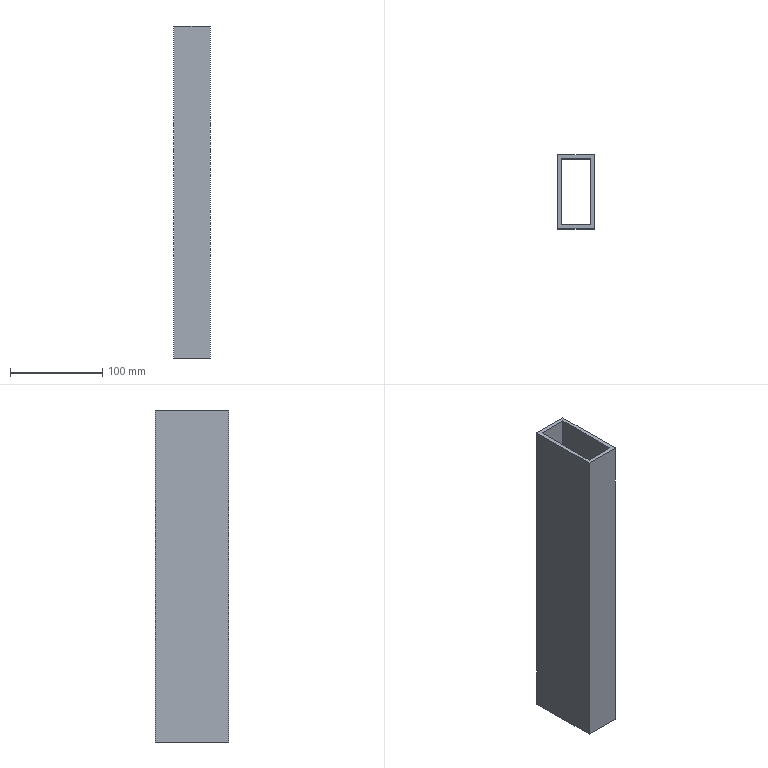Part | SolidWorks | features Extrusion 1 | 1 solid | 10 faces | box 40 x 80 x 360 mm | volume 322560 mm3 | plane 10
STEP:
#1=CARTESIAN_POINT('',(-20.,40.,180.));
#2=VERTEX_POINT('',#1);
#3=CARTESIAN_POINT('',(-20.,-40.,180.));
#4=VERTEX_POINT('',#3);
#5=CARTESIAN_POINT('',(-20.,40.,180.));
#6=DIRECTION('',(0.,-1.,0.));
#7=VECTOR('',#6,1000.);
#8=LINE('',#5,#7);
#9=EDGE_CURVE('',#2,#4,#8,.T.);
#10=ORIENTED_EDGE('',*,*,#9,.F.);
#11=CARTESIAN_POINT('',(-20.,40.,-180.));
#12=VERTEX_POINT('',#11);
#13=CARTESIAN_POINT('',(-20.,40.,-180.));
#14=DIRECTION('',(0.,0.,1.));
#15=VECTOR('',#14,1000.);
#16=LINE('',#13,#15);
#17=EDGE_CURVE('',#12,#2,#16,.T.);
#18=ORIENTED_EDGE('',*,*,#17,.F.);
#19=CARTESIAN_POINT('',(-20.,-40.,-180.));
#20=VERTEX_POINT('',#19);
#21=CARTESIAN_POINT('',(-20.,40.,-180.));
#22=DIRECTION('',(0.,-1.,0.));
#23=VECTOR('',#22,1000.);
#24=LINE('',#21,#23);
#25=EDGE_CURVE('',#12,#20,#24,.T.);
#26=ORIENTED_EDGE('',*,*,#25,.T.);
#27=CARTESIAN_POINT('',(-20.,-40.,-180.));
#28=DIRECTION('',(0.,0.,1.));
#29=VECTOR('',#28,1000.);
#30=LINE('',#27,#29);
#31=EDGE_CURVE('',#20,#4,#30,.T.);
#32=ORIENTED_EDGE('',*,*,#31,.T.);
#33=EDGE_LOOP('',(#10,#18,#26,#32));
#34=FACE_OUTER_BOUND('',#33,.T.);
#35=CARTESIAN_POINT('',(-20.,40.,-180.));
#36=DIRECTION('',(-1.,0.,0.));
#37=DIRECTION('',(0.,0.,1.));
#38=AXIS2_PLACEMENT_3D('',#35,#36,#37);
#39=PLANE('',#38);
#40=ADVANCED_FACE('',(#34),#39,.T.);
#41=CARTESIAN_POINT('',(20.,40.,180.));
#42=VERTEX_POINT('',#41);
#43=CARTESIAN_POINT('',(20.,40.,180.));
#44=DIRECTION('',(-1.,0.,0.));
#45=VECTOR('',#44,1000.);
#46=LINE('',#43,#45);
#47=EDGE_CURVE('',#42,#2,#46,.T.);
#48=ORIENTED_EDGE('',*,*,#47,.F.);
#49=CARTESIAN_POINT('',(20.,40.,-180.));
#50=VERTEX_POINT('',#49);
#51=CARTESIAN_POINT('',(20.,40.,-180.));
#52=DIRECTION('',(0.,0.,1.));
#53=VECTOR('',#52,1000.);
#54=LINE('',#51,#53);
#55=EDGE_CURVE('',#50,#42,#54,.T.);
#56=ORIENTED_EDGE('',*,*,#55,.F.);
#57=CARTESIAN_POINT('',(20.,40.,-180.));
#58=DIRECTION('',(-1.,0.,0.));
#59=VECTOR('',#58,1000.);
#60=LINE('',#57,#59);
#61=EDGE_CURVE('',#50,#12,#60,.T.);
#62=ORIENTED_EDGE('',*,*,#61,.T.);
#63=ORIENTED_EDGE('',*,*,#17,.T.);
#64=EDGE_LOOP('',(#48,#56,#62,#63));
#65=FACE_OUTER_BOUND('',#64,.T.);
#66=CARTESIAN_POINT('',(20.,40.,-180.));
#67=DIRECTION('',(0.,1.,0.));
#68=DIRECTION('',(0.,0.,1.));
#69=AXIS2_PLACEMENT_3D('',#66,#67,#68);
#70=PLANE('',#69);
#71=ADVANCED_FACE('',(#65),#70,.T.);
#72=CARTESIAN_POINT('',(20.,-40.,180.));
#73=VERTEX_POINT('',#72);
#74=CARTESIAN_POINT('',(20.,-40.,180.));
#75=DIRECTION('',(0.,1.,0.));
#76=VECTOR('',#75,1000.);
#77=LINE('',#74,#76);
#78=EDGE_CURVE('',#73,#42,#77,.T.);
#79=ORIENTED_EDGE('',*,*,#78,.F.);
#80=CARTESIAN_POINT('',(20.,-40.,-180.));
#81=VERTEX_POINT('',#80);
#82=CARTESIAN_POINT('',(20.,-40.,-180.));
#83=DIRECTION('',(0.,0.,1.));
#84=VECTOR('',#83,1000.);
#85=LINE('',#82,#84);
#86=EDGE_CURVE('',#81,#73,#85,.T.);
#87=ORIENTED_EDGE('',*,*,#86,.F.);
#88=CARTESIAN_POINT('',(20.,-40.,-180.));
#89=DIRECTION('',(0.,1.,0.));
#90=VECTOR('',#89,1000.);
#91=LINE('',#88,#90);
#92=EDGE_CURVE('',#81,#50,#91,.T.);
#93=ORIENTED_EDGE('',*,*,#92,.T.);
#94=ORIENTED_EDGE('',*,*,#55,.T.);
#95=EDGE_LOOP('',(#79,#87,#93,#94));
#96=FACE_OUTER_BOUND('',#95,.T.);
#97=CARTESIAN_POINT('',(20.,-40.,-180.));
#98=DIRECTION('',(1.,0.,0.));
#99=DIRECTION('',(0.,0.,-1.));
#100=AXIS2_PLACEMENT_3D('',#97,#98,#99);
#101=PLANE('',#100);
#102=ADVANCED_FACE('',(#96),#101,.T.);
#103=CARTESIAN_POINT('',(-20.,-40.,180.));
#104=DIRECTION('',(1.,0.,0.));
#105=VECTOR('',#104,1000.);
#106=LINE('',#103,#105);
#107=EDGE_CURVE('',#4,#73,#106,.T.);
#108=ORIENTED_EDGE('',*,*,#107,.F.);
#109=ORIENTED_EDGE('',*,*,#31,.F.);
#110=CARTESIAN_POINT('',(-20.,-40.,-180.));
#111=DIRECTION('',(1.,0.,0.));
#112=VECTOR('',#111,1000.);
#113=LINE('',#110,#112);
#114=EDGE_CURVE('',#20,#81,#113,.T.);
#115=ORIENTED_EDGE('',*,*,#114,.T.);
#116=ORIENTED_EDGE('',*,*,#86,.T.);
#117=EDGE_LOOP('',(#108,#109,#115,#116));
#118=FACE_OUTER_BOUND('',#117,.T.);
#119=CARTESIAN_POINT('',(-20.,-40.,-180.));
#120=DIRECTION('',(0.,-1.,0.));
#121=DIRECTION('',(0.,0.,-1.));
#122=AXIS2_PLACEMENT_3D('',#119,#120,#121);
#123=PLANE('',#122);
#124=ADVANCED_FACE('',(#118),#123,.T.);
#125=CARTESIAN_POINT('',(16.,36.,-180.));
#126=VERTEX_POINT('',#125);
#127=CARTESIAN_POINT('',(-16.,36.,-180.));
#128=VERTEX_POINT('',#127);
#129=CARTESIAN_POINT('',(16.,36.,-180.));
#130=DIRECTION('',(-1.,0.,0.));
#131=VECTOR('',#130,1000.);
#132=LINE('',#129,#131);
#133=EDGE_CURVE('',#126,#128,#132,.T.);
#134=ORIENTED_EDGE('',*,*,#133,.T.);
#135=CARTESIAN_POINT('',(-16.,-36.,-180.));
#136=VERTEX_POINT('',#135);
#137=CARTESIAN_POINT('',(-16.,36.,-180.));
#138=DIRECTION('',(0.,-1.,0.));
#139=VECTOR('',#138,1000.);
#140=LINE('',#137,#139);
#141=EDGE_CURVE('',#128,#136,#140,.T.);
#142=ORIENTED_EDGE('',*,*,#141,.T.);
#143=CARTESIAN_POINT('',(16.,-36.,-180.));
#144=VERTEX_POINT('',#143);
#145=CARTESIAN_POINT('',(-16.,-36.,-180.));
#146=DIRECTION('',(1.,0.,0.));
#147=VECTOR('',#146,1000.);
#148=LINE('',#145,#147);
#149=EDGE_CURVE('',#136,#144,#148,.T.);
#150=ORIENTED_EDGE('',*,*,#149,.T.);
#151=CARTESIAN_POINT('',(16.,-36.,-180.));
#152=DIRECTION('',(0.,1.,0.));
#153=VECTOR('',#152,1000.);
#154=LINE('',#151,#153);
#155=EDGE_CURVE('',#144,#126,#154,.T.);
#156=ORIENTED_EDGE('',*,*,#155,.T.);
#157=EDGE_LOOP('',(#134,#142,#150,#156));
#158=FACE_BOUND('',#157,.T.);
#159=ORIENTED_EDGE('',*,*,#25,.F.);
#160=ORIENTED_EDGE('',*,*,#61,.F.);
#161=ORIENTED_EDGE('',*,*,#92,.F.);
#162=ORIENTED_EDGE('',*,*,#114,.F.);
#163=EDGE_LOOP('',(#159,#160,#161,#162));
#164=FACE_OUTER_BOUND('',#163,.T.);
#165=CARTESIAN_POINT('',(0.,0.,-180.));
#166=DIRECTION('',(0.,0.,1.));
#167=DIRECTION('',(1.,0.,0.));
#168=AXIS2_PLACEMENT_3D('',#165,#166,#167);
#169=PLANE('',#168);
#170=ADVANCED_FACE('',(#158,#164),#169,.F.);
#171=CARTESIAN_POINT('',(-16.,36.,180.));
#172=VERTEX_POINT('',#171);
#173=CARTESIAN_POINT('',(-16.,-36.,180.));
#174=VERTEX_POINT('',#173);
#175=CARTESIAN_POINT('',(-16.,36.,180.));
#176=DIRECTION('',(0.,-1.,0.));
#177=VECTOR('',#176,1000.);
#178=LINE('',#175,#177);
#179=EDGE_CURVE('',#172,#174,#178,.T.);
#180=ORIENTED_EDGE('',*,*,#179,.F.);
#181=CARTESIAN_POINT('',(16.,36.,180.));
#182=VERTEX_POINT('',#181);
#183=CARTESIAN_POINT('',(16.,36.,180.));
#184=DIRECTION('',(-1.,0.,0.));
#185=VECTOR('',#184,1000.);
#186=LINE('',#183,#185);
#187=EDGE_CURVE('',#182,#172,#186,.T.);
#188=ORIENTED_EDGE('',*,*,#187,.F.);
#189=CARTESIAN_POINT('',(16.,-36.,180.));
#190=VERTEX_POINT('',#189);
#191=CARTESIAN_POINT('',(16.,-36.,180.));
#192=DIRECTION('',(0.,1.,0.));
#193=VECTOR('',#192,1000.);
#194=LINE('',#191,#193);
#195=EDGE_CURVE('',#190,#182,#194,.T.);
#196=ORIENTED_EDGE('',*,*,#195,.F.);
#197=CARTESIAN_POINT('',(-16.,-36.,180.));
#198=DIRECTION('',(1.,0.,0.));
#199=VECTOR('',#198,1000.);
#200=LINE('',#197,#199);
#201=EDGE_CURVE('',#174,#190,#200,.T.);
#202=ORIENTED_EDGE('',*,*,#201,.F.);
#203=EDGE_LOOP('',(#180,#188,#196,#202));
#204=FACE_BOUND('',#203,.T.);
#205=ORIENTED_EDGE('',*,*,#9,.T.);
#206=ORIENTED_EDGE('',*,*,#107,.T.);
#207=ORIENTED_EDGE('',*,*,#78,.T.);
#208=ORIENTED_EDGE('',*,*,#47,.T.);
#209=EDGE_LOOP('',(#205,#206,#207,#208));
#210=FACE_OUTER_BOUND('',#209,.T.);
#211=CARTESIAN_POINT('',(0.,0.,180.));
#212=DIRECTION('',(0.,0.,1.));
#213=DIRECTION('',(1.,0.,0.));
#214=AXIS2_PLACEMENT_3D('',#211,#212,#213);
#215=PLANE('',#214);
#216=ADVANCED_FACE('',(#204,#210),#215,.T.);
#217=ORIENTED_EDGE('',*,*,#179,.T.);
#218=CARTESIAN_POINT('',(-16.,-36.,-180.));
#219=DIRECTION('',(0.,0.,1.));
#220=VECTOR('',#219,1000.);
#221=LINE('',#218,#220);
#222=EDGE_CURVE('',#136,#174,#221,.T.);
#223=ORIENTED_EDGE('',*,*,#222,.F.);
#224=ORIENTED_EDGE('',*,*,#141,.F.);
#225=CARTESIAN_POINT('',(-16.,36.,-180.));
#226=DIRECTION('',(0.,0.,1.));
#227=VECTOR('',#226,1000.);
#228=LINE('',#225,#227);
#229=EDGE_CURVE('',#128,#172,#228,.T.);
#230=ORIENTED_EDGE('',*,*,#229,.T.);
#231=EDGE_LOOP('',(#217,#223,#224,#230));
#232=FACE_OUTER_BOUND('',#231,.T.);
#233=CARTESIAN_POINT('',(-16.,36.,-180.));
#234=DIRECTION('',(-1.,0.,0.));
#235=DIRECTION('',(0.,0.,1.));
#236=AXIS2_PLACEMENT_3D('',#233,#234,#235);
#237=PLANE('',#236);
#238=ADVANCED_FACE('',(#232),#237,.F.);
#239=ORIENTED_EDGE('',*,*,#187,.T.);
#240=ORIENTED_EDGE('',*,*,#229,.F.);
#241=ORIENTED_EDGE('',*,*,#133,.F.);
#242=CARTESIAN_POINT('',(16.,36.,-180.));
#243=DIRECTION('',(0.,0.,1.));
#244=VECTOR('',#243,1000.);
#245=LINE('',#242,#244);
#246=EDGE_CURVE('',#126,#182,#245,.T.);
#247=ORIENTED_EDGE('',*,*,#246,.T.);
#248=EDGE_LOOP('',(#239,#240,#241,#247));
#249=FACE_OUTER_BOUND('',#248,.T.);
#250=CARTESIAN_POINT('',(16.,36.,-180.));
#251=DIRECTION('',(0.,1.,0.));
#252=DIRECTION('',(0.,0.,1.));
#253=AXIS2_PLACEMENT_3D('',#250,#251,#252);
#254=PLANE('',#253);
#255=ADVANCED_FACE('',(#249),#254,.F.);
#256=ORIENTED_EDGE('',*,*,#195,.T.);
#257=ORIENTED_EDGE('',*,*,#246,.F.);
#258=ORIENTED_EDGE('',*,*,#155,.F.);
#259=CARTESIAN_POINT('',(16.,-36.,-180.));
#260=DIRECTION('',(0.,0.,1.));
#261=VECTOR('',#260,1000.);
#262=LINE('',#259,#261);
#263=EDGE_CURVE('',#144,#190,#262,.T.);
#264=ORIENTED_EDGE('',*,*,#263,.T.);
#265=EDGE_LOOP('',(#256,#257,#258,#264));
#266=FACE_OUTER_BOUND('',#265,.T.);
#267=CARTESIAN_POINT('',(16.,-36.,-180.));
#268=DIRECTION('',(1.,0.,0.));
#269=DIRECTION('',(0.,0.,-1.));
#270=AXIS2_PLACEMENT_3D('',#267,#268,#269);
#271=PLANE('',#270);
#272=ADVANCED_FACE('',(#266),#271,.F.);
#273=ORIENTED_EDGE('',*,*,#201,.T.);
#274=ORIENTED_EDGE('',*,*,#263,.F.);
#275=ORIENTED_EDGE('',*,*,#149,.F.);
#276=ORIENTED_EDGE('',*,*,#222,.T.);
#277=EDGE_LOOP('',(#273,#274,#275,#276));
#278=FACE_OUTER_BOUND('',#277,.T.);
#279=CARTESIAN_POINT('',(-16.,-36.,-180.));
#280=DIRECTION('',(0.,-1.,0.));
#281=DIRECTION('',(0.,0.,-1.));
#282=AXIS2_PLACEMENT_3D('',#279,#280,#281);
#283=PLANE('',#282);
#284=ADVANCED_FACE('',(#278),#283,.F.);
#285=CLOSED_SHELL('',(#40,#71,#102,#124,#170,#216,#238,#255,#272,#284));
#286=MANIFOLD_SOLID_BREP('',#285);
#287=CARTESIAN_POINT('',(0.,0.,0.));
#288=DIRECTION('',(0.,0.,1.));
#289=DIRECTION('',(1.,0.,0.));
#290=AXIS2_PLACEMENT_3D('',#287,#288,#289);
#291=(LENGTH_UNIT()NAMED_UNIT(*)SI_UNIT(.MILLI.,.METRE.));
#292=UNCERTAINTY_MEASURE_WITH_UNIT(LENGTH_MEASURE(0.00001),#291,'','');
#293=(NAMED_UNIT(*)PLANE_ANGLE_UNIT()SI_UNIT($,.RADIAN.));
#294=(NAMED_UNIT(*)SI_UNIT($,.STERADIAN.)SOLID_ANGLE_UNIT());
#295=(GEOMETRIC_REPRESENTATION_CONTEXT(3)GLOBAL_UNCERTAINTY_ASSIGNED_CONTEXT((#292))GLOBAL_UNIT_ASSIGNED_CONTEXT((#291,#293,#294))REPRESENTATION_CONTEXT('',''));
#296=ADVANCED_BREP_SHAPE_REPRESENTATION('',(#286,#290),#295);